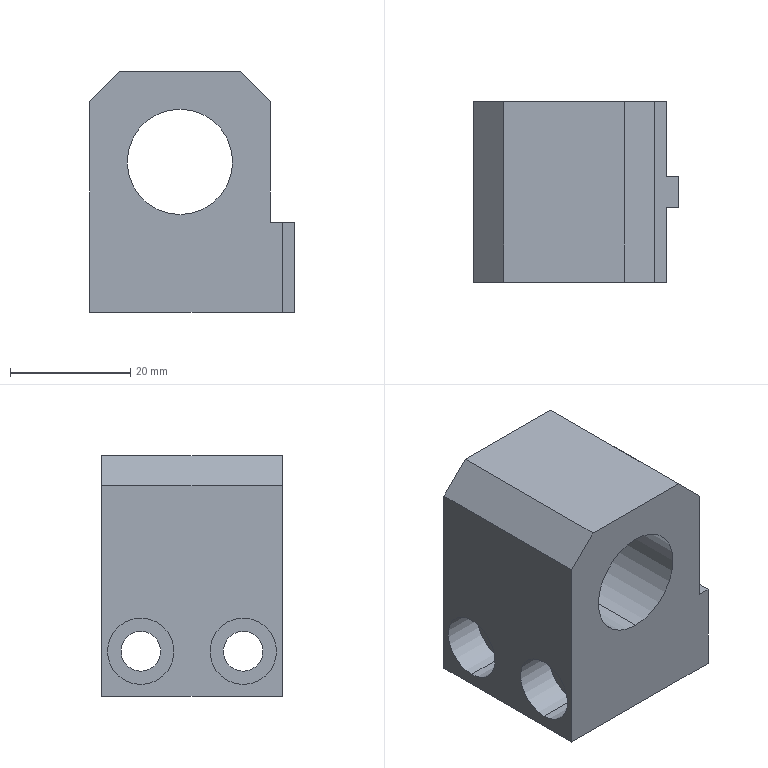Part | SolidWorks | features BaseBody 1 | 1 solid | 26 faces | box 34 x 30 x 40 mm | volume 26067 mm3 | plane 16 | cylinder 10 | commonest cylinder face diameters 6.6 x4 11 x4 17.5 x2
STEP:
#1=CARTESIAN_POINT('',(-34.,30.,35.));
#2=VERTEX_POINT('',#1);
#3=CARTESIAN_POINT('',(-29.,30.,40.));
#4=VERTEX_POINT('',#3);
#5=CARTESIAN_POINT('',(-29.,30.,40.));
#6=DIRECTION('',(0.7071,0.,0.7071));
#7=VECTOR('',#6,1000.);
#8=LINE('',#5,#7);
#9=EDGE_CURVE('',#2,#4,#8,.T.);
#10=ORIENTED_EDGE('',*,*,#9,.F.);
#11=CARTESIAN_POINT('',(-34.,0.,35.));
#12=VERTEX_POINT('',#11);
#13=CARTESIAN_POINT('',(-34.,30.,35.));
#14=DIRECTION('',(0.,1.,0.));
#15=VECTOR('',#14,1000.);
#16=LINE('',#13,#15);
#17=EDGE_CURVE('',#12,#2,#16,.T.);
#18=ORIENTED_EDGE('',*,*,#17,.F.);
#19=CARTESIAN_POINT('',(-29.,0.,40.));
#20=VERTEX_POINT('',#19);
#21=CARTESIAN_POINT('',(-34.5,0.,34.5));
#22=DIRECTION('',(-0.7071,0.,-0.7071));
#23=VECTOR('',#22,1000.);
#24=LINE('',#21,#23);
#25=EDGE_CURVE('',#20,#12,#24,.T.);
#26=ORIENTED_EDGE('',*,*,#25,.F.);
#27=CARTESIAN_POINT('',(-29.,30.,40.));
#28=DIRECTION('',(0.,-1.,0.));
#29=VECTOR('',#28,1000.);
#30=LINE('',#27,#29);
#31=EDGE_CURVE('',#4,#20,#30,.T.);
#32=ORIENTED_EDGE('',*,*,#31,.F.);
#33=EDGE_LOOP('',(#10,#18,#26,#32));
#34=FACE_OUTER_BOUND('',#33,.T.);
#35=CARTESIAN_POINT('',(-29.,30.,40.));
#36=DIRECTION('',(0.7071,0.,-0.7071));
#37=DIRECTION('',(0.,-1.,0.));
#38=AXIS2_PLACEMENT_3D('',#35,#36,#37);
#39=PLANE('',#38);
#40=ADVANCED_FACE('',(#34),#39,.F.);
#41=CARTESIAN_POINT('',(-9.,30.,40.));
#42=VERTEX_POINT('',#41);
#43=CARTESIAN_POINT('',(-4.,30.,35.));
#44=VERTEX_POINT('',#43);
#45=CARTESIAN_POINT('',(-4.,30.,35.));
#46=DIRECTION('',(0.7071,0.,-0.7071));
#47=VECTOR('',#46,1000.);
#48=LINE('',#45,#47);
#49=EDGE_CURVE('',#42,#44,#48,.T.);
#50=ORIENTED_EDGE('',*,*,#49,.F.);
#51=CARTESIAN_POINT('',(-9.,0.,40.));
#52=VERTEX_POINT('',#51);
#53=CARTESIAN_POINT('',(-9.,30.,40.));
#54=DIRECTION('',(0.,1.,0.));
#55=VECTOR('',#54,1000.);
#56=LINE('',#53,#55);
#57=EDGE_CURVE('',#52,#42,#56,.T.);
#58=ORIENTED_EDGE('',*,*,#57,.F.);
#59=CARTESIAN_POINT('',(-4.,0.,35.));
#60=VERTEX_POINT('',#59);
#61=CARTESIAN_POINT('',(15.5,0.,15.5));
#62=DIRECTION('',(-0.7071,0.,0.7071));
#63=VECTOR('',#62,1000.);
#64=LINE('',#61,#63);
#65=EDGE_CURVE('',#60,#52,#64,.T.);
#66=ORIENTED_EDGE('',*,*,#65,.F.);
#67=CARTESIAN_POINT('',(-4.,30.,35.));
#68=DIRECTION('',(0.,-1.,0.));
#69=VECTOR('',#68,1000.);
#70=LINE('',#67,#69);
#71=EDGE_CURVE('',#44,#60,#70,.T.);
#72=ORIENTED_EDGE('',*,*,#71,.F.);
#73=EDGE_LOOP('',(#50,#58,#66,#72));
#74=FACE_OUTER_BOUND('',#73,.T.);
#75=CARTESIAN_POINT('',(-4.,30.,35.));
#76=DIRECTION('',(-0.7071,0.,-0.7071));
#77=DIRECTION('',(-0.7071,0.,0.7071));
#78=AXIS2_PLACEMENT_3D('',#75,#76,#77);
#79=PLANE('',#78);
#80=ADVANCED_FACE('',(#74),#79,.F.);
#81=CARTESIAN_POINT('',(-27.2,23.5,2.));
#82=VERTEX_POINT('',#81);
#83=CARTESIAN_POINT('',(-34.,23.5,2.));
#84=VERTEX_POINT('',#83);
#85=CARTESIAN_POINT('',(-34.,23.5,2.));
#86=DIRECTION('',(-1.,0.,0.));
#87=VECTOR('',#86,1000.);
#88=LINE('',#85,#87);
#89=EDGE_CURVE('',#82,#84,#88,.T.);
#90=ORIENTED_EDGE('',*,*,#89,.F.);
#91=CARTESIAN_POINT('',(-27.2,23.5,13.));
#92=VERTEX_POINT('',#91);
#93=CARTESIAN_POINT('',(-27.2,23.5,7.5));
#94=DIRECTION('',(-1.,0.,0.));
#95=DIRECTION('',(0.,0.,1.));
#96=AXIS2_PLACEMENT_3D('',#93,#94,#95);
#97=CIRCLE('',#96,5.5);
#98=EDGE_CURVE('',#92,#82,#97,.T.);
#99=ORIENTED_EDGE('',*,*,#98,.F.);
#100=CARTESIAN_POINT('',(-34.,23.5,13.));
#101=VERTEX_POINT('',#100);
#102=CARTESIAN_POINT('',(-34.,23.5,13.));
#103=DIRECTION('',(-1.,0.,0.));
#104=VECTOR('',#103,1000.);
#105=LINE('',#102,#104);
#106=EDGE_CURVE('',#92,#101,#105,.T.);
#107=ORIENTED_EDGE('',*,*,#106,.T.);
#108=CARTESIAN_POINT('',(-34.,23.5,7.5));
#109=DIRECTION('',(-1.,0.,0.));
#110=DIRECTION('',(0.,0.,1.));
#111=AXIS2_PLACEMENT_3D('',#108,#109,#110);
#112=CIRCLE('',#111,5.5);
#113=EDGE_CURVE('',#101,#84,#112,.T.);
#114=ORIENTED_EDGE('',*,*,#113,.T.);
#115=EDGE_LOOP('',(#90,#99,#107,#114));
#116=FACE_OUTER_BOUND('',#115,.T.);
#117=CARTESIAN_POINT('',(-34.,23.5,7.5));
#118=DIRECTION('',(-1.,0.,0.));
#119=DIRECTION('',(0.,0.,1.));
#120=AXIS2_PLACEMENT_3D('',#117,#118,#119);
#121=CYLINDRICAL_SURFACE('',#120,5.5);
#122=ADVANCED_FACE('',(#116),#121,.F.);
#123=CARTESIAN_POINT('',(-27.2,23.5,10.8));
#124=VERTEX_POINT('',#123);
#125=CARTESIAN_POINT('',(-27.2,23.5,4.2));
#126=VERTEX_POINT('',#125);
#127=CARTESIAN_POINT('',(-27.2,23.5,7.5));
#128=DIRECTION('',(-1.,0.,0.));
#129=DIRECTION('',(0.,0.,1.));
#130=AXIS2_PLACEMENT_3D('',#127,#128,#129);
#131=CIRCLE('',#130,3.3);
#132=EDGE_CURVE('',#124,#126,#131,.T.);
#133=ORIENTED_EDGE('',*,*,#132,.F.);
#134=CARTESIAN_POINT('',(-27.2,23.5,7.5));
#135=DIRECTION('',(-1.,0.,0.));
#136=DIRECTION('',(0.,0.,1.));
#137=AXIS2_PLACEMENT_3D('',#134,#135,#136);
#138=CIRCLE('',#137,3.3);
#139=EDGE_CURVE('',#126,#124,#138,.T.);
#140=ORIENTED_EDGE('',*,*,#139,.F.);
#141=EDGE_LOOP('',(#133,#140));
#142=FACE_BOUND('',#141,.T.);
#143=ORIENTED_EDGE('',*,*,#98,.T.);
#144=CARTESIAN_POINT('',(-27.2,23.5,7.5));
#145=DIRECTION('',(-1.,0.,0.));
#146=DIRECTION('',(0.,0.,1.));
#147=AXIS2_PLACEMENT_3D('',#144,#145,#146);
#148=CIRCLE('',#147,5.5);
#149=EDGE_CURVE('',#82,#92,#148,.T.);
#150=ORIENTED_EDGE('',*,*,#149,.T.);
#151=EDGE_LOOP('',(#143,#150));
#152=FACE_OUTER_BOUND('',#151,.T.);
#153=CARTESIAN_POINT('',(-27.2,26.8,7.5));
#154=DIRECTION('',(1.,0.,0.));
#155=DIRECTION('',(0.,0.,-1.));
#156=AXIS2_PLACEMENT_3D('',#153,#154,#155);
#157=PLANE('',#156);
#158=ADVANCED_FACE('',(#142,#152),#157,.F.);
#159=CARTESIAN_POINT('',(-2.,23.5,4.2));
#160=VERTEX_POINT('',#159);
#161=CARTESIAN_POINT('',(-34.,23.5,4.2));
#162=DIRECTION('',(-1.,0.,0.));
#163=VECTOR('',#162,1000.);
#164=LINE('',#161,#163);
#165=EDGE_CURVE('',#160,#126,#164,.T.);
#166=ORIENTED_EDGE('',*,*,#165,.F.);
#167=CARTESIAN_POINT('',(-2.,23.5,10.8));
#168=VERTEX_POINT('',#167);
#169=CARTESIAN_POINT('',(-2.,23.5,7.5));
#170=DIRECTION('',(1.,0.,0.));
#171=DIRECTION('',(0.,0.,-1.));
#172=AXIS2_PLACEMENT_3D('',#169,#170,#171);
#173=CIRCLE('',#172,3.3);
#174=EDGE_CURVE('',#160,#168,#173,.T.);
#175=ORIENTED_EDGE('',*,*,#174,.T.);
#176=CARTESIAN_POINT('',(-34.,23.5,10.8));
#177=DIRECTION('',(-1.,0.,0.));
#178=VECTOR('',#177,1000.);
#179=LINE('',#176,#178);
#180=EDGE_CURVE('',#168,#124,#179,.T.);
#181=ORIENTED_EDGE('',*,*,#180,.T.);
#182=ORIENTED_EDGE('',*,*,#132,.T.);
#183=EDGE_LOOP('',(#166,#175,#181,#182));
#184=FACE_OUTER_BOUND('',#183,.T.);
#185=CARTESIAN_POINT('',(-34.,23.5,7.5));
#186=DIRECTION('',(-1.,0.,0.));
#187=DIRECTION('',(0.,0.,1.));
#188=AXIS2_PLACEMENT_3D('',#185,#186,#187);
#189=CYLINDRICAL_SURFACE('',#188,3.3);
#190=ADVANCED_FACE('',(#184),#189,.F.);
#191=CARTESIAN_POINT('',(-27.2,6.5,2.));
#192=VERTEX_POINT('',#191);
#193=CARTESIAN_POINT('',(-34.,6.5,2.));
#194=VERTEX_POINT('',#193);
#195=CARTESIAN_POINT('',(-34.,6.5,2.));
#196=DIRECTION('',(-1.,0.,0.));
#197=VECTOR('',#196,1000.);
#198=LINE('',#195,#197);
#199=EDGE_CURVE('',#192,#194,#198,.T.);
#200=ORIENTED_EDGE('',*,*,#199,.F.);
#201=CARTESIAN_POINT('',(-27.2,6.5,13.));
#202=VERTEX_POINT('',#201);
#203=CARTESIAN_POINT('',(-27.2,6.5,7.5));
#204=DIRECTION('',(-1.,0.,0.));
#205=DIRECTION('',(0.,0.,1.));
#206=AXIS2_PLACEMENT_3D('',#203,#204,#205);
#207=CIRCLE('',#206,5.5);
#208=EDGE_CURVE('',#202,#192,#207,.T.);
#209=ORIENTED_EDGE('',*,*,#208,.F.);
#210=CARTESIAN_POINT('',(-34.,6.5,13.));
#211=VERTEX_POINT('',#210);
#212=CARTESIAN_POINT('',(-34.,6.5,13.));
#213=DIRECTION('',(-1.,0.,0.));
#214=VECTOR('',#213,1000.);
#215=LINE('',#212,#214);
#216=EDGE_CURVE('',#202,#211,#215,.T.);
#217=ORIENTED_EDGE('',*,*,#216,.T.);
#218=CARTESIAN_POINT('',(-34.,6.5,7.5));
#219=DIRECTION('',(-1.,0.,0.));
#220=DIRECTION('',(0.,0.,1.));
#221=AXIS2_PLACEMENT_3D('',#218,#219,#220);
#222=CIRCLE('',#221,5.5);
#223=EDGE_CURVE('',#211,#194,#222,.T.);
#224=ORIENTED_EDGE('',*,*,#223,.T.);
#225=EDGE_LOOP('',(#200,#209,#217,#224));
#226=FACE_OUTER_BOUND('',#225,.T.);
#227=CARTESIAN_POINT('',(-34.,6.5,7.5));
#228=DIRECTION('',(-1.,0.,0.));
#229=DIRECTION('',(0.,0.,1.));
#230=AXIS2_PLACEMENT_3D('',#227,#228,#229);
#231=CYLINDRICAL_SURFACE('',#230,5.5);
#232=ADVANCED_FACE('',(#226),#231,.F.);
#233=CARTESIAN_POINT('',(-27.2,6.5,10.8));
#234=VERTEX_POINT('',#233);
#235=CARTESIAN_POINT('',(-27.2,6.5,4.2));
#236=VERTEX_POINT('',#235);
#237=CARTESIAN_POINT('',(-27.2,6.5,7.5));
#238=DIRECTION('',(-1.,0.,0.));
#239=DIRECTION('',(0.,0.,1.));
#240=AXIS2_PLACEMENT_3D('',#237,#238,#239);
#241=CIRCLE('',#240,3.3);
#242=EDGE_CURVE('',#234,#236,#241,.T.);
#243=ORIENTED_EDGE('',*,*,#242,.F.);
#244=CARTESIAN_POINT('',(-27.2,6.5,7.5));
#245=DIRECTION('',(-1.,0.,0.));
#246=DIRECTION('',(0.,0.,1.));
#247=AXIS2_PLACEMENT_3D('',#244,#245,#246);
#248=CIRCLE('',#247,3.3);
#249=EDGE_CURVE('',#236,#234,#248,.T.);
#250=ORIENTED_EDGE('',*,*,#249,.F.);
#251=EDGE_LOOP('',(#243,#250));
#252=FACE_BOUND('',#251,.T.);
#253=ORIENTED_EDGE('',*,*,#208,.T.);
#254=CARTESIAN_POINT('',(-27.2,6.5,7.5));
#255=DIRECTION('',(-1.,0.,0.));
#256=DIRECTION('',(0.,0.,1.));
#257=AXIS2_PLACEMENT_3D('',#254,#255,#256);
#258=CIRCLE('',#257,5.5);
#259=EDGE_CURVE('',#192,#202,#258,.T.);
#260=ORIENTED_EDGE('',*,*,#259,.T.);
#261=EDGE_LOOP('',(#253,#260));
#262=FACE_OUTER_BOUND('',#261,.T.);
#263=CARTESIAN_POINT('',(-27.2,9.8,7.5));
#264=DIRECTION('',(1.,0.,0.));
#265=DIRECTION('',(0.,0.,-1.));
#266=AXIS2_PLACEMENT_3D('',#263,#264,#265);
#267=PLANE('',#266);
#268=ADVANCED_FACE('',(#252,#262),#267,.F.);
#269=CARTESIAN_POINT('',(-2.,6.5,4.2));
#270=VERTEX_POINT('',#269);
#271=CARTESIAN_POINT('',(-34.,6.5,4.2));
#272=DIRECTION('',(-1.,0.,0.));
#273=VECTOR('',#272,1000.);
#274=LINE('',#271,#273);
#275=EDGE_CURVE('',#270,#236,#274,.T.);
#276=ORIENTED_EDGE('',*,*,#275,.F.);
#277=CARTESIAN_POINT('',(-2.,6.5,10.8));
#278=VERTEX_POINT('',#277);
#279=CARTESIAN_POINT('',(-2.,6.5,7.5));
#280=DIRECTION('',(1.,0.,0.));
#281=DIRECTION('',(0.,0.,-1.));
#282=AXIS2_PLACEMENT_3D('',#279,#280,#281);
#283=CIRCLE('',#282,3.3);
#284=EDGE_CURVE('',#270,#278,#283,.T.);
#285=ORIENTED_EDGE('',*,*,#284,.T.);
#286=CARTESIAN_POINT('',(-34.,6.5,10.8));
#287=DIRECTION('',(-1.,0.,0.));
#288=VECTOR('',#287,1000.);
#289=LINE('',#286,#288);
#290=EDGE_CURVE('',#278,#234,#289,.T.);
#291=ORIENTED_EDGE('',*,*,#290,.T.);
#292=ORIENTED_EDGE('',*,*,#242,.T.);
#293=EDGE_LOOP('',(#276,#285,#291,#292));
#294=FACE_OUTER_BOUND('',#293,.T.);
#295=CARTESIAN_POINT('',(-34.,6.5,7.5));
#296=DIRECTION('',(-1.,0.,0.));
#297=DIRECTION('',(0.,0.,1.));
#298=AXIS2_PLACEMENT_3D('',#295,#296,#297);
#299=CYLINDRICAL_SURFACE('',#298,3.3);
#300=ADVANCED_FACE('',(#294),#299,.F.);
#301=CARTESIAN_POINT('',(-2.,23.5,7.5));
#302=DIRECTION('',(1.,0.,0.));
#303=DIRECTION('',(0.,0.,-1.));
#304=AXIS2_PLACEMENT_3D('',#301,#302,#303);
#305=CIRCLE('',#304,3.3);
#306=EDGE_CURVE('',#168,#160,#305,.T.);
#307=ORIENTED_EDGE('',*,*,#306,.F.);
#308=ORIENTED_EDGE('',*,*,#174,.F.);
#309=EDGE_LOOP('',(#307,#308));
#310=FACE_BOUND('',#309,.T.);
#311=CARTESIAN_POINT('',(-2.,30.,15.));
#312=VERTEX_POINT('',#311);
#313=CARTESIAN_POINT('',(-2.,17.5,15.));
#314=VERTEX_POINT('',#313);
#315=CARTESIAN_POINT('',(-2.,30.,15.));
#316=DIRECTION('',(0.,-1.,0.));
#317=VECTOR('',#316,1000.);
#318=LINE('',#315,#317);
#319=EDGE_CURVE('',#312,#314,#318,.T.);
#320=ORIENTED_EDGE('',*,*,#319,.T.);
#321=CARTESIAN_POINT('',(-2.,17.5,0.));
#322=VERTEX_POINT('',#321);
#323=CARTESIAN_POINT('',(-2.,17.5,15.));
#324=DIRECTION('',(0.,0.,-1.));
#325=VECTOR('',#324,1000.);
#326=LINE('',#323,#325);
#327=EDGE_CURVE('',#314,#322,#326,.T.);
#328=ORIENTED_EDGE('',*,*,#327,.T.);
#329=CARTESIAN_POINT('',(-2.,30.,0.));
#330=VERTEX_POINT('',#329);
#331=CARTESIAN_POINT('',(-2.,30.,0.));
#332=DIRECTION('',(0.,1.,0.));
#333=VECTOR('',#332,1000.);
#334=LINE('',#331,#333);
#335=EDGE_CURVE('',#322,#330,#334,.T.);
#336=ORIENTED_EDGE('',*,*,#335,.T.);
#337=CARTESIAN_POINT('',(-2.,30.,15.));
#338=DIRECTION('',(0.,0.,1.));
#339=VECTOR('',#338,1000.);
#340=LINE('',#337,#339);
#341=EDGE_CURVE('',#330,#312,#340,.T.);
#342=ORIENTED_EDGE('',*,*,#341,.T.);
#343=EDGE_LOOP('',(#320,#328,#336,#342));
#344=FACE_OUTER_BOUND('',#343,.T.);
#345=CARTESIAN_POINT('',(-2.,0.,0.));
#346=DIRECTION('',(1.,0.,0.));
#347=DIRECTION('',(0.,0.,-1.));
#348=AXIS2_PLACEMENT_3D('',#345,#346,#347);
#349=PLANE('',#348);
#350=ADVANCED_FACE('',(#310,#344),#349,.T.);
#351=CARTESIAN_POINT('',(0.,17.5,15.));
#352=VERTEX_POINT('',#351);
#353=CARTESIAN_POINT('',(0.,17.5,0.));
#354=VERTEX_POINT('',#353);
#355=CARTESIAN_POINT('',(0.,17.5,15.));
#356=DIRECTION('',(0.,0.,-1.));
#357=VECTOR('',#356,1000.);
#358=LINE('',#355,#357);
#359=EDGE_CURVE('',#352,#354,#358,.T.);
#360=ORIENTED_EDGE('',*,*,#359,.T.);
#361=CARTESIAN_POINT('',(-2.,17.5,0.));
#362=DIRECTION('',(1.,0.,0.));
#363=VECTOR('',#362,1000.);
#364=LINE('',#361,#363);
#365=EDGE_CURVE('',#322,#354,#364,.T.);
#366=ORIENTED_EDGE('',*,*,#365,.F.);
#367=ORIENTED_EDGE('',*,*,#327,.F.);
#368=CARTESIAN_POINT('',(-2.,17.5,15.));
#369=DIRECTION('',(1.,0.,0.));
#370=VECTOR('',#369,1000.);
#371=LINE('',#368,#370);
#372=EDGE_CURVE('',#314,#352,#371,.T.);
#373=ORIENTED_EDGE('',*,*,#372,.T.);
#374=EDGE_LOOP('',(#360,#366,#367,#373));
#375=FACE_OUTER_BOUND('',#374,.T.);
#376=CARTESIAN_POINT('',(-2.,17.5,15.));
#377=DIRECTION('',(0.,-1.,0.));
#378=DIRECTION('',(0.,0.,-1.));
#379=AXIS2_PLACEMENT_3D('',#376,#377,#378);
#380=PLANE('',#379);
#381=ADVANCED_FACE('',(#375),#380,.F.);
#382=CARTESIAN_POINT('',(-2.,6.5,7.5));
#383=DIRECTION('',(1.,0.,0.));
#384=DIRECTION('',(0.,0.,-1.));
#385=AXIS2_PLACEMENT_3D('',#382,#383,#384);
#386=CIRCLE('',#385,3.3);
#387=EDGE_CURVE('',#278,#270,#386,.T.);
#388=ORIENTED_EDGE('',*,*,#387,.F.);
#389=ORIENTED_EDGE('',*,*,#284,.F.);
#390=EDGE_LOOP('',(#388,#389));
#391=FACE_BOUND('',#390,.T.);
#392=CARTESIAN_POINT('',(-2.,0.,15.));
#393=VERTEX_POINT('',#392);
#394=CARTESIAN_POINT('',(-2.,0.,0.));
#395=VERTEX_POINT('',#394);
#396=CARTESIAN_POINT('',(-2.,0.,15.));
#397=DIRECTION('',(0.,0.,-1.));
#398=VECTOR('',#397,1000.);
#399=LINE('',#396,#398);
#400=EDGE_CURVE('',#393,#395,#399,.T.);
#401=ORIENTED_EDGE('',*,*,#400,.T.);
#402=CARTESIAN_POINT('',(-2.,12.5,0.));
#403=VERTEX_POINT('',#402);
#404=CARTESIAN_POINT('',(-2.,0.,0.));
#405=DIRECTION('',(0.,1.,0.));
#406=VECTOR('',#405,1000.);
#407=LINE('',#404,#406);
#408=EDGE_CURVE('',#395,#403,#407,.T.);
#409=ORIENTED_EDGE('',*,*,#408,.T.);
#410=CARTESIAN_POINT('',(-2.,12.5,15.));
#411=VERTEX_POINT('',#410);
#412=CARTESIAN_POINT('',(-2.,12.5,15.));
#413=DIRECTION('',(0.,0.,1.));
#414=VECTOR('',#413,1000.);
#415=LINE('',#412,#414);
#416=EDGE_CURVE('',#403,#411,#415,.T.);
#417=ORIENTED_EDGE('',*,*,#416,.T.);
#418=CARTESIAN_POINT('',(-2.,0.,15.));
#419=DIRECTION('',(0.,-1.,0.));
#420=VECTOR('',#419,1000.);
#421=LINE('',#418,#420);
#422=EDGE_CURVE('',#411,#393,#421,.T.);
#423=ORIENTED_EDGE('',*,*,#422,.T.);
#424=EDGE_LOOP('',(#401,#409,#417,#423));
#425=FACE_OUTER_BOUND('',#424,.T.);
#426=CARTESIAN_POINT('',(-2.,0.,0.));
#427=DIRECTION('',(1.,0.,0.));
#428=DIRECTION('',(0.,0.,-1.));
#429=AXIS2_PLACEMENT_3D('',#426,#427,#428);
#430=PLANE('',#429);
#431=ADVANCED_FACE('',(#391,#425),#430,.T.);
#432=CARTESIAN_POINT('',(0.,12.5,0.));
#433=VERTEX_POINT('',#432);
#434=CARTESIAN_POINT('',(0.,12.5,15.));
#435=VERTEX_POINT('',#434);
#436=CARTESIAN_POINT('',(0.,12.5,15.));
#437=DIRECTION('',(0.,0.,1.));
#438=VECTOR('',#437,1000.);
#439=LINE('',#436,#438);
#440=EDGE_CURVE('',#433,#435,#439,.T.);
#441=ORIENTED_EDGE('',*,*,#440,.T.);
#442=CARTESIAN_POINT('',(-2.,12.5,15.));
#443=DIRECTION('',(1.,0.,0.));
#444=VECTOR('',#443,1000.);
#445=LINE('',#442,#444);
#446=EDGE_CURVE('',#411,#435,#445,.T.);
#447=ORIENTED_EDGE('',*,*,#446,.F.);
#448=ORIENTED_EDGE('',*,*,#416,.F.);
#449=CARTESIAN_POINT('',(-2.,12.5,0.));
#450=DIRECTION('',(1.,0.,0.));
#451=VECTOR('',#450,1000.);
#452=LINE('',#449,#451);
#453=EDGE_CURVE('',#403,#433,#452,.T.);
#454=ORIENTED_EDGE('',*,*,#453,.T.);
#455=EDGE_LOOP('',(#441,#447,#448,#454));
#456=FACE_OUTER_BOUND('',#455,.T.);
#457=CARTESIAN_POINT('',(-2.,12.5,15.));
#458=DIRECTION('',(0.,1.,0.));
#459=DIRECTION('',(0.,0.,-1.));
#460=AXIS2_PLACEMENT_3D('',#457,#458,#459);
#461=PLANE('',#460);
#462=ADVANCED_FACE('',(#456),#461,.F.);
#463=CARTESIAN_POINT('',(-19.,0.,16.25));
#464=VERTEX_POINT('',#463);
#465=CARTESIAN_POINT('',(-19.,30.,16.25));
#466=VERTEX_POINT('',#465);
#467=CARTESIAN_POINT('',(-19.,30.,16.25));
#468=DIRECTION('',(0.,1.,0.));
#469=VECTOR('',#468,1000.);
#470=LINE('',#467,#469);
#471=EDGE_CURVE('',#464,#466,#470,.T.);
#472=ORIENTED_EDGE('',*,*,#471,.F.);
#473=CARTESIAN_POINT('',(-19.,0.,33.75));
#474=VERTEX_POINT('',#473);
#475=CARTESIAN_POINT('',(-19.,0.,25.));
#476=DIRECTION('',(0.,1.,0.));
#477=DIRECTION('',(0.,0.,1.));
#478=AXIS2_PLACEMENT_3D('',#475,#476,#477);
#479=CIRCLE('',#478,8.75);
#480=EDGE_CURVE('',#474,#464,#479,.T.);
#481=ORIENTED_EDGE('',*,*,#480,.F.);
#482=CARTESIAN_POINT('',(-19.,30.,33.75));
#483=VERTEX_POINT('',#482);
#484=CARTESIAN_POINT('',(-19.,30.,33.75));
#485=DIRECTION('',(0.,1.,0.));
#486=VECTOR('',#485,1000.);
#487=LINE('',#484,#486);
#488=EDGE_CURVE('',#474,#483,#487,.T.);
#489=ORIENTED_EDGE('',*,*,#488,.T.);
#490=CARTESIAN_POINT('',(-19.,30.,25.));
#491=DIRECTION('',(0.,1.,0.));
#492=DIRECTION('',(0.,0.,1.));
#493=AXIS2_PLACEMENT_3D('',#490,#491,#492);
#494=CIRCLE('',#493,8.75);
#495=EDGE_CURVE('',#483,#466,#494,.T.);
#496=ORIENTED_EDGE('',*,*,#495,.T.);
#497=EDGE_LOOP('',(#472,#481,#489,#496));
#498=FACE_OUTER_BOUND('',#497,.T.);
#499=CARTESIAN_POINT('',(-19.,30.,25.));
#500=DIRECTION('',(0.,1.,0.));
#501=DIRECTION('',(0.,0.,1.));
#502=AXIS2_PLACEMENT_3D('',#499,#500,#501);
#503=CYLINDRICAL_SURFACE('',#502,8.75);
#504=ADVANCED_FACE('',(#498),#503,.F.);
#505=CARTESIAN_POINT('',(0.,30.,15.));
#506=DIRECTION('',(0.,-1.,0.));
#507=VECTOR('',#506,1000.);
#508=LINE('',#505,#507);
#509=EDGE_CURVE('',#352,#435,#508,.T.);
#510=ORIENTED_EDGE('',*,*,#509,.F.);
#511=ORIENTED_EDGE('',*,*,#372,.F.);
#512=ORIENTED_EDGE('',*,*,#319,.F.);
#513=CARTESIAN_POINT('',(-4.,30.,15.));
#514=VERTEX_POINT('',#513);
#515=CARTESIAN_POINT('',(0.,30.,15.));
#516=DIRECTION('',(1.,0.,0.));
#517=VECTOR('',#516,1000.);
#518=LINE('',#515,#517);
#519=EDGE_CURVE('',#514,#312,#518,.T.);
#520=ORIENTED_EDGE('',*,*,#519,.F.);
#521=CARTESIAN_POINT('',(-4.,0.,15.));
#522=VERTEX_POINT('',#521);
#523=CARTESIAN_POINT('',(-4.,30.,15.));
#524=DIRECTION('',(0.,-1.,0.));
#525=VECTOR('',#524,1000.);
#526=LINE('',#523,#525);
#527=EDGE_CURVE('',#514,#522,#526,.T.);
#528=ORIENTED_EDGE('',*,*,#527,.T.);
#529=CARTESIAN_POINT('',(0.,0.,15.));
#530=DIRECTION('',(1.,0.,0.));
#531=VECTOR('',#530,1000.);
#532=LINE('',#529,#531);
#533=EDGE_CURVE('',#522,#393,#532,.T.);
#534=ORIENTED_EDGE('',*,*,#533,.T.);
#535=ORIENTED_EDGE('',*,*,#422,.F.);
#536=ORIENTED_EDGE('',*,*,#446,.T.);
#537=EDGE_LOOP('',(#510,#511,#512,#520,#528,#534,#535,#536));
#538=FACE_OUTER_BOUND('',#537,.T.);
#539=CARTESIAN_POINT('',(0.,30.,15.));
#540=DIRECTION('',(0.,0.,-1.));
#541=DIRECTION('',(0.,-1.,0.));
#542=AXIS2_PLACEMENT_3D('',#539,#540,#541);
#543=PLANE('',#542);
#544=ADVANCED_FACE('',(#538),#543,.F.);
#545=CARTESIAN_POINT('',(-4.,30.,15.));
#546=DIRECTION('',(0.,0.,-1.));
#547=VECTOR('',#546,1000.);
#548=LINE('',#545,#547);
#549=EDGE_CURVE('',#44,#514,#548,.T.);
#550=ORIENTED_EDGE('',*,*,#549,.F.);
#551=ORIENTED_EDGE('',*,*,#71,.T.);
#552=CARTESIAN_POINT('',(-4.,0.,15.));
#553=DIRECTION('',(0.,0.,-1.));
#554=VECTOR('',#553,1000.);
#555=LINE('',#552,#554);
#556=EDGE_CURVE('',#60,#522,#555,.T.);
#557=ORIENTED_EDGE('',*,*,#556,.T.);
#558=ORIENTED_EDGE('',*,*,#527,.F.);
#559=EDGE_LOOP('',(#550,#551,#557,#558));
#560=FACE_OUTER_BOUND('',#559,.T.);
#561=CARTESIAN_POINT('',(-4.,30.,15.));
#562=DIRECTION('',(-1.,0.,0.));
#563=DIRECTION('',(0.,1.,0.));
#564=AXIS2_PLACEMENT_3D('',#561,#562,#563);
#565=PLANE('',#564);
#566=ADVANCED_FACE('',(#560),#565,.F.);
#567=CARTESIAN_POINT('',(-34.,0.,40.));
#568=DIRECTION('',(1.,0.,0.));
#569=VECTOR('',#568,1000.);
#570=LINE('',#567,#569);
#571=EDGE_CURVE('',#20,#52,#570,.T.);
#572=ORIENTED_EDGE('',*,*,#571,.T.);
#573=ORIENTED_EDGE('',*,*,#57,.T.);
#574=CARTESIAN_POINT('',(-34.,30.,40.));
#575=DIRECTION('',(1.,0.,0.));
#576=VECTOR('',#575,1000.);
#577=LINE('',#574,#576);
#578=EDGE_CURVE('',#4,#42,#577,.T.);
#579=ORIENTED_EDGE('',*,*,#578,.F.);
#580=ORIENTED_EDGE('',*,*,#31,.T.);
#581=EDGE_LOOP('',(#572,#573,#579,#580));
#582=FACE_OUTER_BOUND('',#581,.T.);
#583=CARTESIAN_POINT('',(-34.,30.,40.));
#584=DIRECTION('',(0.,0.,-1.));
#585=DIRECTION('',(0.,-1.,0.));
#586=AXIS2_PLACEMENT_3D('',#583,#584,#585);
#587=PLANE('',#586);
#588=ADVANCED_FACE('',(#582),#587,.F.);
#589=ORIENTED_EDGE('',*,*,#223,.F.);
#590=CARTESIAN_POINT('',(-34.,6.5,7.5));
#591=DIRECTION('',(-1.,0.,0.));
#592=DIRECTION('',(0.,0.,1.));
#593=AXIS2_PLACEMENT_3D('',#590,#591,#592);
#594=CIRCLE('',#593,5.5);
#595=EDGE_CURVE('',#194,#211,#594,.T.);
#596=ORIENTED_EDGE('',*,*,#595,.F.);
#597=EDGE_LOOP('',(#589,#596));
#598=FACE_BOUND('',#597,.T.);
#599=ORIENTED_EDGE('',*,*,#113,.F.);
#600=CARTESIAN_POINT('',(-34.,23.5,7.5));
#601=DIRECTION('',(-1.,0.,0.));
#602=DIRECTION('',(0.,0.,1.));
#603=AXIS2_PLACEMENT_3D('',#600,#601,#602);
#604=CIRCLE('',#603,5.5);
#605=EDGE_CURVE('',#84,#101,#604,.T.);
#606=ORIENTED_EDGE('',*,*,#605,.F.);
#607=EDGE_LOOP('',(#599,#606));
#608=FACE_BOUND('',#607,.T.);
#609=CARTESIAN_POINT('',(-34.,0.,0.));
#610=VERTEX_POINT('',#609);
#611=CARTESIAN_POINT('',(-34.,0.,0.));
#612=DIRECTION('',(0.,0.,1.));
#613=VECTOR('',#612,1000.);
#614=LINE('',#611,#613);
#615=EDGE_CURVE('',#610,#12,#614,.T.);
#616=ORIENTED_EDGE('',*,*,#615,.T.);
#617=ORIENTED_EDGE('',*,*,#17,.T.);
#618=CARTESIAN_POINT('',(-34.,30.,0.));
#619=VERTEX_POINT('',#618);
#620=CARTESIAN_POINT('',(-34.,30.,0.));
#621=DIRECTION('',(0.,0.,1.));
#622=VECTOR('',#621,1000.);
#623=LINE('',#620,#622);
#624=EDGE_CURVE('',#619,#2,#623,.T.);
#625=ORIENTED_EDGE('',*,*,#624,.F.);
#626=CARTESIAN_POINT('',(-34.,30.,0.));
#627=DIRECTION('',(0.,-1.,0.));
#628=VECTOR('',#627,1000.);
#629=LINE('',#626,#628);
#630=EDGE_CURVE('',#619,#610,#629,.T.);
#631=ORIENTED_EDGE('',*,*,#630,.T.);
#632=EDGE_LOOP('',(#616,#617,#625,#631));
#633=FACE_OUTER_BOUND('',#632,.T.);
#634=CARTESIAN_POINT('',(-34.,30.,0.));
#635=DIRECTION('',(1.,0.,0.));
#636=DIRECTION('',(0.,0.,-1.));
#637=AXIS2_PLACEMENT_3D('',#634,#635,#636);
#638=PLANE('',#637);
#639=ADVANCED_FACE('',(#598,#608,#633),#638,.F.);
#640=ORIENTED_EDGE('',*,*,#335,.F.);
#641=ORIENTED_EDGE('',*,*,#365,.T.);
#642=CARTESIAN_POINT('',(0.,30.,0.));
#643=DIRECTION('',(0.,-1.,0.));
#644=VECTOR('',#643,1000.);
#645=LINE('',#642,#644);
#646=EDGE_CURVE('',#354,#433,#645,.T.);
#647=ORIENTED_EDGE('',*,*,#646,.T.);
#648=ORIENTED_EDGE('',*,*,#453,.F.);
#649=ORIENTED_EDGE('',*,*,#408,.F.);
#650=CARTESIAN_POINT('',(-34.,0.,0.));
#651=DIRECTION('',(-1.,0.,0.));
#652=VECTOR('',#651,1000.);
#653=LINE('',#650,#652);
#654=EDGE_CURVE('',#395,#610,#653,.T.);
#655=ORIENTED_EDGE('',*,*,#654,.T.);
#656=ORIENTED_EDGE('',*,*,#630,.F.);
#657=CARTESIAN_POINT('',(-34.,30.,0.));
#658=DIRECTION('',(-1.,0.,0.));
#659=VECTOR('',#658,1000.);
#660=LINE('',#657,#659);
#661=EDGE_CURVE('',#330,#619,#660,.T.);
#662=ORIENTED_EDGE('',*,*,#661,.F.);
#663=EDGE_LOOP('',(#640,#641,#647,#648,#649,#655,#656,#662));
#664=FACE_OUTER_BOUND('',#663,.T.);
#665=CARTESIAN_POINT('',(-34.,30.,0.));
#666=DIRECTION('',(0.,0.,1.));
#667=DIRECTION('',(1.,0.,0.));
#668=AXIS2_PLACEMENT_3D('',#665,#666,#667);
#669=PLANE('',#668);
#670=ADVANCED_FACE('',(#664),#669,.F.);
#671=ORIENTED_EDGE('',*,*,#646,.F.);
#672=ORIENTED_EDGE('',*,*,#359,.F.);
#673=ORIENTED_EDGE('',*,*,#509,.T.);
#674=ORIENTED_EDGE('',*,*,#440,.F.);
#675=EDGE_LOOP('',(#671,#672,#673,#674));
#676=FACE_OUTER_BOUND('',#675,.T.);
#677=CARTESIAN_POINT('',(0.,30.,0.));
#678=DIRECTION('',(-1.,0.,0.));
#679=DIRECTION('',(0.,1.,0.));
#680=AXIS2_PLACEMENT_3D('',#677,#678,#679);
#681=PLANE('',#680);
#682=ADVANCED_FACE('',(#676),#681,.F.);
#683=ORIENTED_EDGE('',*,*,#480,.T.);
#684=CARTESIAN_POINT('',(-19.,0.,25.));
#685=DIRECTION('',(0.,1.,0.));
#686=DIRECTION('',(0.,0.,1.));
#687=AXIS2_PLACEMENT_3D('',#684,#685,#686);
#688=CIRCLE('',#687,8.75);
#689=EDGE_CURVE('',#464,#474,#688,.T.);
#690=ORIENTED_EDGE('',*,*,#689,.T.);
#691=EDGE_LOOP('',(#683,#690));
#692=FACE_BOUND('',#691,.T.);
#693=ORIENTED_EDGE('',*,*,#556,.F.);
#694=ORIENTED_EDGE('',*,*,#65,.T.);
#695=ORIENTED_EDGE('',*,*,#571,.F.);
#696=ORIENTED_EDGE('',*,*,#25,.T.);
#697=ORIENTED_EDGE('',*,*,#615,.F.);
#698=ORIENTED_EDGE('',*,*,#654,.F.);
#699=ORIENTED_EDGE('',*,*,#400,.F.);
#700=ORIENTED_EDGE('',*,*,#533,.F.);
#701=EDGE_LOOP('',(#693,#694,#695,#696,#697,#698,#699,#700));
#702=FACE_OUTER_BOUND('',#701,.T.);
#703=CARTESIAN_POINT('',(0.,0.,0.));
#704=DIRECTION('',(0.,-1.,0.));
#705=DIRECTION('',(0.,0.,-1.));
#706=AXIS2_PLACEMENT_3D('',#703,#704,#705);
#707=PLANE('',#706);
#708=ADVANCED_FACE('',(#692,#702),#707,.T.);
#709=ORIENTED_EDGE('',*,*,#495,.F.);
#710=CARTESIAN_POINT('',(-19.,30.,25.));
#711=DIRECTION('',(0.,1.,0.));
#712=DIRECTION('',(0.,0.,1.));
#713=AXIS2_PLACEMENT_3D('',#710,#711,#712);
#714=CIRCLE('',#713,8.75);
#715=EDGE_CURVE('',#466,#483,#714,.T.);
#716=ORIENTED_EDGE('',*,*,#715,.F.);
#717=EDGE_LOOP('',(#709,#716));
#718=FACE_BOUND('',#717,.T.);
#719=ORIENTED_EDGE('',*,*,#578,.T.);
#720=ORIENTED_EDGE('',*,*,#49,.T.);
#721=ORIENTED_EDGE('',*,*,#549,.T.);
#722=ORIENTED_EDGE('',*,*,#519,.T.);
#723=ORIENTED_EDGE('',*,*,#341,.F.);
#724=ORIENTED_EDGE('',*,*,#661,.T.);
#725=ORIENTED_EDGE('',*,*,#624,.T.);
#726=ORIENTED_EDGE('',*,*,#9,.T.);
#727=EDGE_LOOP('',(#719,#720,#721,#722,#723,#724,#725,#726));
#728=FACE_OUTER_BOUND('',#727,.T.);
#729=CARTESIAN_POINT('',(0.,30.,0.));
#730=DIRECTION('',(0.,-1.,0.));
#731=DIRECTION('',(0.,0.,-1.));
#732=AXIS2_PLACEMENT_3D('',#729,#730,#731);
#733=PLANE('',#732);
#734=ADVANCED_FACE('',(#718,#728),#733,.F.);
#735=ORIENTED_EDGE('',*,*,#689,.F.);
#736=ORIENTED_EDGE('',*,*,#471,.T.);
#737=ORIENTED_EDGE('',*,*,#715,.T.);
#738=ORIENTED_EDGE('',*,*,#488,.F.);
#739=EDGE_LOOP('',(#735,#736,#737,#738));
#740=FACE_OUTER_BOUND('',#739,.T.);
#741=CARTESIAN_POINT('',(-19.,30.,25.));
#742=DIRECTION('',(0.,1.,0.));
#743=DIRECTION('',(0.,0.,1.));
#744=AXIS2_PLACEMENT_3D('',#741,#742,#743);
#745=CYLINDRICAL_SURFACE('',#744,8.75);
#746=ADVANCED_FACE('',(#740),#745,.F.);
#747=ORIENTED_EDGE('',*,*,#387,.T.);
#748=ORIENTED_EDGE('',*,*,#275,.T.);
#749=ORIENTED_EDGE('',*,*,#249,.T.);
#750=ORIENTED_EDGE('',*,*,#290,.F.);
#751=EDGE_LOOP('',(#747,#748,#749,#750));
#752=FACE_OUTER_BOUND('',#751,.T.);
#753=CARTESIAN_POINT('',(-34.,6.5,7.5));
#754=DIRECTION('',(-1.,0.,0.));
#755=DIRECTION('',(0.,0.,1.));
#756=AXIS2_PLACEMENT_3D('',#753,#754,#755);
#757=CYLINDRICAL_SURFACE('',#756,3.3);
#758=ADVANCED_FACE('',(#752),#757,.F.);
#759=ORIENTED_EDGE('',*,*,#259,.F.);
#760=ORIENTED_EDGE('',*,*,#199,.T.);
#761=ORIENTED_EDGE('',*,*,#595,.T.);
#762=ORIENTED_EDGE('',*,*,#216,.F.);
#763=EDGE_LOOP('',(#759,#760,#761,#762));
#764=FACE_OUTER_BOUND('',#763,.T.);
#765=CARTESIAN_POINT('',(-34.,6.5,7.5));
#766=DIRECTION('',(-1.,0.,0.));
#767=DIRECTION('',(0.,0.,1.));
#768=AXIS2_PLACEMENT_3D('',#765,#766,#767);
#769=CYLINDRICAL_SURFACE('',#768,5.5);
#770=ADVANCED_FACE('',(#764),#769,.F.);
#771=ORIENTED_EDGE('',*,*,#306,.T.);
#772=ORIENTED_EDGE('',*,*,#165,.T.);
#773=ORIENTED_EDGE('',*,*,#139,.T.);
#774=ORIENTED_EDGE('',*,*,#180,.F.);
#775=EDGE_LOOP('',(#771,#772,#773,#774));
#776=FACE_OUTER_BOUND('',#775,.T.);
#777=CARTESIAN_POINT('',(-34.,23.5,7.5));
#778=DIRECTION('',(-1.,0.,0.));
#779=DIRECTION('',(0.,0.,1.));
#780=AXIS2_PLACEMENT_3D('',#777,#778,#779);
#781=CYLINDRICAL_SURFACE('',#780,3.3);
#782=ADVANCED_FACE('',(#776),#781,.F.);
#783=ORIENTED_EDGE('',*,*,#149,.F.);
#784=ORIENTED_EDGE('',*,*,#89,.T.);
#785=ORIENTED_EDGE('',*,*,#605,.T.);
#786=ORIENTED_EDGE('',*,*,#106,.F.);
#787=EDGE_LOOP('',(#783,#784,#785,#786));
#788=FACE_OUTER_BOUND('',#787,.T.);
#789=CARTESIAN_POINT('',(-34.,23.5,7.5));
#790=DIRECTION('',(-1.,0.,0.));
#791=DIRECTION('',(0.,0.,1.));
#792=AXIS2_PLACEMENT_3D('',#789,#790,#791);
#793=CYLINDRICAL_SURFACE('',#792,5.5);
#794=ADVANCED_FACE('',(#788),#793,.F.);
#795=CLOSED_SHELL('',(#40,#80,#122,#158,#190,#232,#268,#300,#350,#381,#431,#462,#504,#544,#566,#588,#639,#670,#682,#708,#734,#746,#758,#770,#782,#794));
#796=MANIFOLD_SOLID_BREP('',#795);
#797=CARTESIAN_POINT('',(0.,0.,0.));
#798=DIRECTION('',(0.,0.,1.));
#799=DIRECTION('',(1.,0.,0.));
#800=AXIS2_PLACEMENT_3D('',#797,#798,#799);
#801=(LENGTH_UNIT()NAMED_UNIT(*)SI_UNIT(.MILLI.,.METRE.));
#802=UNCERTAINTY_MEASURE_WITH_UNIT(LENGTH_MEASURE(0.00001),#801,'','');
#803=(NAMED_UNIT(*)PLANE_ANGLE_UNIT()SI_UNIT($,.RADIAN.));
#804=(NAMED_UNIT(*)SI_UNIT($,.STERADIAN.)SOLID_ANGLE_UNIT());
#805=(GEOMETRIC_REPRESENTATION_CONTEXT(3)GLOBAL_UNCERTAINTY_ASSIGNED_CONTEXT((#802))GLOBAL_UNIT_ASSIGNED_CONTEXT((#801,#803,#804))REPRESENTATION_CONTEXT('',''));
#806=ADVANCED_BREP_SHAPE_REPRESENTATION('',(#796,#800),#805);